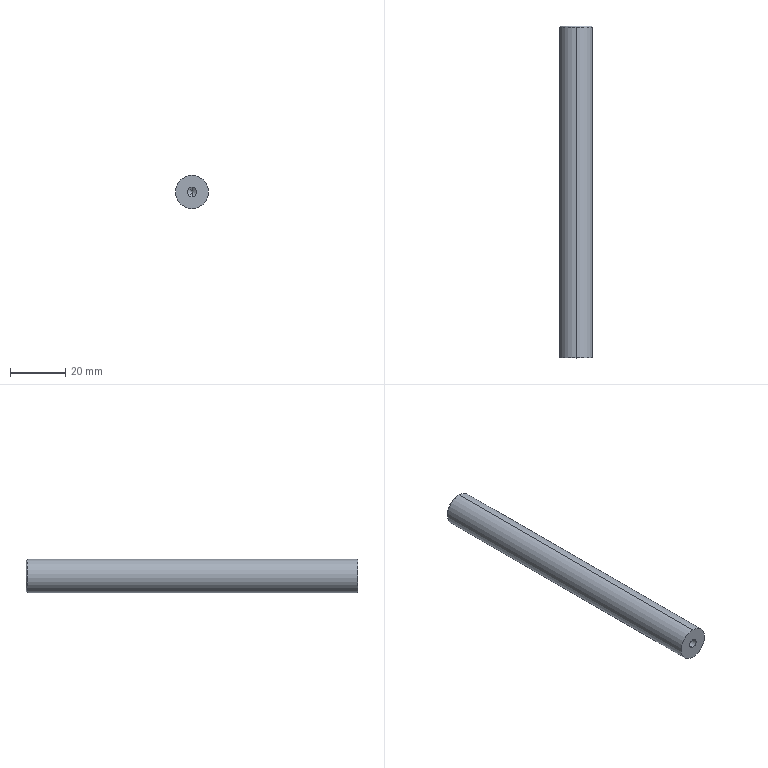Part | SolidWorks | features Chamfer 1, Extrusion 1, HoleWzd 1, ICE 1 | 1 solid | 10 faces | box 12 x 120 x 12 mm | volume 13432 mm3 | cone 4 | cylinder 4 | plane 2 | commonest cylinder face diameters 3.3 x2 12 x2
STEP:
#1=CARTESIAN_POINT('',(0.,120.,5.5));
#2=VERTEX_POINT('',#1);
#3=CARTESIAN_POINT('',(0.,120.,-5.5));
#4=VERTEX_POINT('',#3);
#5=CARTESIAN_POINT('',(0.,120.,0.));
#6=DIRECTION('',(0.,1.,0.));
#7=DIRECTION('',(0.,0.,1.));
#8=AXIS2_PLACEMENT_3D('',#5,#6,#7);
#9=CIRCLE('',#8,5.5);
#10=EDGE_CURVE('',#2,#4,#9,.T.);
#11=ORIENTED_EDGE('',*,*,#10,.F.);
#12=CARTESIAN_POINT('',(0.,119.5,6.));
#13=VERTEX_POINT('',#12);
#14=CARTESIAN_POINT('',(0.,120.,5.5));
#15=DIRECTION('',(0.,-0.7071,0.7071));
#16=VECTOR('',#15,1000.);
#17=LINE('',#14,#16);
#18=EDGE_CURVE('',#2,#13,#17,.T.);
#19=ORIENTED_EDGE('',*,*,#18,.T.);
#20=CARTESIAN_POINT('',(0.,119.5,-6.));
#21=VERTEX_POINT('',#20);
#22=CARTESIAN_POINT('',(0.,119.5,0.));
#23=DIRECTION('',(0.,-1.,0.));
#24=DIRECTION('',(0.,0.,1.));
#25=AXIS2_PLACEMENT_3D('',#22,#23,#24);
#26=CIRCLE('',#25,6.);
#27=EDGE_CURVE('',#21,#13,#26,.T.);
#28=ORIENTED_EDGE('',*,*,#27,.F.);
#29=CARTESIAN_POINT('',(0.,120.,-5.5));
#30=DIRECTION('',(0.,-0.7071,-0.7071));
#31=VECTOR('',#30,1000.);
#32=LINE('',#29,#31);
#33=EDGE_CURVE('',#4,#21,#32,.T.);
#34=ORIENTED_EDGE('',*,*,#33,.F.);
#35=EDGE_LOOP('',(#11,#19,#28,#34));
#36=FACE_OUTER_BOUND('',#35,.T.);
#37=CARTESIAN_POINT('',(0.,120.,0.));
#38=DIRECTION('',(0.,-1.,0.));
#39=DIRECTION('',(0.,0.,-1.));
#40=AXIS2_PLACEMENT_3D('',#37,#38,#39);
#41=CONICAL_SURFACE('',#40,5.5,0.7854);
#42=ADVANCED_FACE('',(#36),#41,.T.);
#43=CARTESIAN_POINT('',(0.,15.5,1.65));
#44=VERTEX_POINT('',#43);
#45=CARTESIAN_POINT('',(0.,15.5,-1.65));
#46=VERTEX_POINT('',#45);
#47=CARTESIAN_POINT('',(0.,15.5,0.));
#48=DIRECTION('',(0.,-1.,0.));
#49=DIRECTION('',(0.,0.,-1.));
#50=AXIS2_PLACEMENT_3D('',#47,#48,#49);
#51=CIRCLE('',#50,1.65);
#52=EDGE_CURVE('',#44,#46,#51,.T.);
#53=ORIENTED_EDGE('',*,*,#52,.F.);
#54=CARTESIAN_POINT('',(0.,0.,1.65));
#55=VERTEX_POINT('',#54);
#56=CARTESIAN_POINT('',(0.,0.,1.65));
#57=DIRECTION('',(0.,-1.,0.));
#58=VECTOR('',#57,1000.);
#59=LINE('',#56,#58);
#60=EDGE_CURVE('',#44,#55,#59,.T.);
#61=ORIENTED_EDGE('',*,*,#60,.T.);
#62=CARTESIAN_POINT('',(0.,0.,-1.65));
#63=VERTEX_POINT('',#62);
#64=CARTESIAN_POINT('',(0.,0.,0.));
#65=DIRECTION('',(0.,-1.,0.));
#66=DIRECTION('',(0.,0.,-1.));
#67=AXIS2_PLACEMENT_3D('',#64,#65,#66);
#68=CIRCLE('',#67,1.65);
#69=EDGE_CURVE('',#55,#63,#68,.T.);
#70=ORIENTED_EDGE('',*,*,#69,.T.);
#71=CARTESIAN_POINT('',(0.,0.,-1.65));
#72=DIRECTION('',(0.,-1.,0.));
#73=VECTOR('',#72,1000.);
#74=LINE('',#71,#73);
#75=EDGE_CURVE('',#46,#63,#74,.T.);
#76=ORIENTED_EDGE('',*,*,#75,.F.);
#77=EDGE_LOOP('',(#53,#61,#70,#76));
#78=FACE_OUTER_BOUND('',#77,.T.);
#79=CARTESIAN_POINT('',(0.,0.,0.));
#80=DIRECTION('',(0.,-1.,0.));
#81=DIRECTION('',(0.,0.,-1.));
#82=AXIS2_PLACEMENT_3D('',#79,#80,#81);
#83=CYLINDRICAL_SURFACE('',#82,1.65);
#84=ADVANCED_FACE('',(#78),#83,.F.);
#85=CARTESIAN_POINT('',(0.,16.491,0.));
#86=VERTEX_POINT('',#85);
#87=CARTESIAN_POINT('',(0.,15.5,-1.65));
#88=DIRECTION('',(0.,-0.515,-0.8572));
#89=VECTOR('',#88,1000.);
#90=LINE('',#87,#89);
#91=EDGE_CURVE('',#86,#46,#90,.T.);
#92=ORIENTED_EDGE('',*,*,#91,.F.);
#93=CARTESIAN_POINT('',(0.,15.5,1.65));
#94=DIRECTION('',(0.,-0.515,0.8572));
#95=VECTOR('',#94,1000.);
#96=LINE('',#93,#95);
#97=EDGE_CURVE('',#86,#44,#96,.T.);
#98=ORIENTED_EDGE('',*,*,#97,.T.);
#99=ORIENTED_EDGE('',*,*,#52,.T.);
#100=EDGE_LOOP('',(#92,#98,#99));
#101=FACE_OUTER_BOUND('',#100,.T.);
#102=CARTESIAN_POINT('',(0.,15.5,0.));
#103=DIRECTION('',(0.,-1.,0.));
#104=DIRECTION('',(0.,0.,-1.));
#105=AXIS2_PLACEMENT_3D('',#102,#103,#104);
#106=CONICAL_SURFACE('',#105,1.65,1.03);
#107=ADVANCED_FACE('',(#101),#106,.F.);
#108=ORIENTED_EDGE('',*,*,#27,.T.);
#109=CARTESIAN_POINT('',(0.,0.,6.));
#110=VERTEX_POINT('',#109);
#111=CARTESIAN_POINT('',(0.,120.,6.));
#112=DIRECTION('',(0.,-1.,0.));
#113=VECTOR('',#112,1000.);
#114=LINE('',#111,#113);
#115=EDGE_CURVE('',#13,#110,#114,.T.);
#116=ORIENTED_EDGE('',*,*,#115,.T.);
#117=CARTESIAN_POINT('',(0.,0.,-6.));
#118=VERTEX_POINT('',#117);
#119=CARTESIAN_POINT('',(0.,0.,0.));
#120=DIRECTION('',(0.,1.,0.));
#121=DIRECTION('',(0.,0.,1.));
#122=AXIS2_PLACEMENT_3D('',#119,#120,#121);
#123=CIRCLE('',#122,6.);
#124=EDGE_CURVE('',#110,#118,#123,.T.);
#125=ORIENTED_EDGE('',*,*,#124,.T.);
#126=CARTESIAN_POINT('',(0.,120.,-6.));
#127=DIRECTION('',(0.,-1.,0.));
#128=VECTOR('',#127,1000.);
#129=LINE('',#126,#128);
#130=EDGE_CURVE('',#21,#118,#129,.T.);
#131=ORIENTED_EDGE('',*,*,#130,.F.);
#132=EDGE_LOOP('',(#108,#116,#125,#131));
#133=FACE_OUTER_BOUND('',#132,.T.);
#134=CARTESIAN_POINT('',(0.,120.,0.));
#135=DIRECTION('',(0.,-1.,0.));
#136=DIRECTION('',(0.,0.,-1.));
#137=AXIS2_PLACEMENT_3D('',#134,#135,#136);
#138=CYLINDRICAL_SURFACE('',#137,6.);
#139=ADVANCED_FACE('',(#133),#138,.T.);
#140=ORIENTED_EDGE('',*,*,#115,.F.);
#141=CARTESIAN_POINT('',(0.,119.5,0.));
#142=DIRECTION('',(0.,-1.,0.));
#143=DIRECTION('',(0.,0.,1.));
#144=AXIS2_PLACEMENT_3D('',#141,#142,#143);
#145=CIRCLE('',#144,6.);
#146=EDGE_CURVE('',#13,#21,#145,.T.);
#147=ORIENTED_EDGE('',*,*,#146,.T.);
#148=ORIENTED_EDGE('',*,*,#130,.T.);
#149=CARTESIAN_POINT('',(0.,0.,0.));
#150=DIRECTION('',(0.,1.,0.));
#151=DIRECTION('',(0.,0.,1.));
#152=AXIS2_PLACEMENT_3D('',#149,#150,#151);
#153=CIRCLE('',#152,6.);
#154=EDGE_CURVE('',#118,#110,#153,.T.);
#155=ORIENTED_EDGE('',*,*,#154,.T.);
#156=EDGE_LOOP('',(#140,#147,#148,#155));
#157=FACE_OUTER_BOUND('',#156,.T.);
#158=CARTESIAN_POINT('',(0.,120.,0.));
#159=DIRECTION('',(0.,-1.,0.));
#160=DIRECTION('',(0.,0.,-1.));
#161=AXIS2_PLACEMENT_3D('',#158,#159,#160);
#162=CYLINDRICAL_SURFACE('',#161,6.);
#163=ADVANCED_FACE('',(#157),#162,.T.);
#164=CARTESIAN_POINT('',(0.,120.,0.));
#165=DIRECTION('',(0.,1.,0.));
#166=DIRECTION('',(0.,0.,1.));
#167=AXIS2_PLACEMENT_3D('',#164,#165,#166);
#168=CIRCLE('',#167,5.5);
#169=EDGE_CURVE('',#4,#2,#168,.T.);
#170=ORIENTED_EDGE('',*,*,#169,.T.);
#171=ORIENTED_EDGE('',*,*,#10,.T.);
#172=EDGE_LOOP('',(#170,#171));
#173=FACE_OUTER_BOUND('',#172,.T.);
#174=CARTESIAN_POINT('',(0.,120.,0.));
#175=DIRECTION('',(0.,1.,0.));
#176=DIRECTION('',(0.,0.,1.));
#177=AXIS2_PLACEMENT_3D('',#174,#175,#176);
#178=PLANE('',#177);
#179=ADVANCED_FACE('',(#173),#178,.T.);
#180=CARTESIAN_POINT('',(0.,0.,0.));
#181=DIRECTION('',(0.,-1.,0.));
#182=DIRECTION('',(0.,0.,-1.));
#183=AXIS2_PLACEMENT_3D('',#180,#181,#182);
#184=CIRCLE('',#183,1.65);
#185=EDGE_CURVE('',#63,#55,#184,.T.);
#186=ORIENTED_EDGE('',*,*,#185,.F.);
#187=ORIENTED_EDGE('',*,*,#69,.F.);
#188=EDGE_LOOP('',(#186,#187));
#189=FACE_BOUND('',#188,.T.);
#190=ORIENTED_EDGE('',*,*,#154,.F.);
#191=ORIENTED_EDGE('',*,*,#124,.F.);
#192=EDGE_LOOP('',(#190,#191));
#193=FACE_OUTER_BOUND('',#192,.T.);
#194=CARTESIAN_POINT('',(0.,0.,0.));
#195=DIRECTION('',(0.,1.,0.));
#196=DIRECTION('',(0.,0.,1.));
#197=AXIS2_PLACEMENT_3D('',#194,#195,#196);
#198=PLANE('',#197);
#199=ADVANCED_FACE('',(#189,#193),#198,.F.);
#200=ORIENTED_EDGE('',*,*,#97,.F.);
#201=ORIENTED_EDGE('',*,*,#91,.T.);
#202=CARTESIAN_POINT('',(0.,15.5,0.));
#203=DIRECTION('',(0.,-1.,0.));
#204=DIRECTION('',(0.,0.,-1.));
#205=AXIS2_PLACEMENT_3D('',#202,#203,#204);
#206=CIRCLE('',#205,1.65);
#207=EDGE_CURVE('',#46,#44,#206,.T.);
#208=ORIENTED_EDGE('',*,*,#207,.T.);
#209=EDGE_LOOP('',(#200,#201,#208));
#210=FACE_OUTER_BOUND('',#209,.T.);
#211=CARTESIAN_POINT('',(0.,15.5,0.));
#212=DIRECTION('',(0.,-1.,0.));
#213=DIRECTION('',(0.,0.,-1.));
#214=AXIS2_PLACEMENT_3D('',#211,#212,#213);
#215=CONICAL_SURFACE('',#214,1.65,1.03);
#216=ADVANCED_FACE('',(#210),#215,.F.);
#217=ORIENTED_EDGE('',*,*,#60,.F.);
#218=ORIENTED_EDGE('',*,*,#207,.F.);
#219=ORIENTED_EDGE('',*,*,#75,.T.);
#220=ORIENTED_EDGE('',*,*,#185,.T.);
#221=EDGE_LOOP('',(#217,#218,#219,#220));
#222=FACE_OUTER_BOUND('',#221,.T.);
#223=CARTESIAN_POINT('',(0.,0.,0.));
#224=DIRECTION('',(0.,-1.,0.));
#225=DIRECTION('',(0.,0.,-1.));
#226=AXIS2_PLACEMENT_3D('',#223,#224,#225);
#227=CYLINDRICAL_SURFACE('',#226,1.65);
#228=ADVANCED_FACE('',(#222),#227,.F.);
#229=ORIENTED_EDGE('',*,*,#18,.F.);
#230=ORIENTED_EDGE('',*,*,#169,.F.);
#231=ORIENTED_EDGE('',*,*,#33,.T.);
#232=ORIENTED_EDGE('',*,*,#146,.F.);
#233=EDGE_LOOP('',(#229,#230,#231,#232));
#234=FACE_OUTER_BOUND('',#233,.T.);
#235=CARTESIAN_POINT('',(0.,120.,0.));
#236=DIRECTION('',(0.,-1.,0.));
#237=DIRECTION('',(0.,0.,-1.));
#238=AXIS2_PLACEMENT_3D('',#235,#236,#237);
#239=CONICAL_SURFACE('',#238,5.5,0.7854);
#240=ADVANCED_FACE('',(#234),#239,.T.);
#241=CLOSED_SHELL('',(#42,#84,#107,#139,#163,#179,#199,#216,#228,#240));
#242=MANIFOLD_SOLID_BREP('',#241);
#243=CARTESIAN_POINT('',(0.,0.,0.));
#244=DIRECTION('',(0.,0.,1.));
#245=DIRECTION('',(1.,0.,0.));
#246=AXIS2_PLACEMENT_3D('',#243,#244,#245);
#247=(LENGTH_UNIT()NAMED_UNIT(*)SI_UNIT(.MILLI.,.METRE.));
#248=UNCERTAINTY_MEASURE_WITH_UNIT(LENGTH_MEASURE(0.00001),#247,'','');
#249=(NAMED_UNIT(*)PLANE_ANGLE_UNIT()SI_UNIT($,.RADIAN.));
#250=(NAMED_UNIT(*)SI_UNIT($,.STERADIAN.)SOLID_ANGLE_UNIT());
#251=(GEOMETRIC_REPRESENTATION_CONTEXT(3)GLOBAL_UNCERTAINTY_ASSIGNED_CONTEXT((#248))GLOBAL_UNIT_ASSIGNED_CONTEXT((#247,#249,#250))REPRESENTATION_CONTEXT('',''));
#252=ADVANCED_BREP_SHAPE_REPRESENTATION('',(#242,#246),#251);